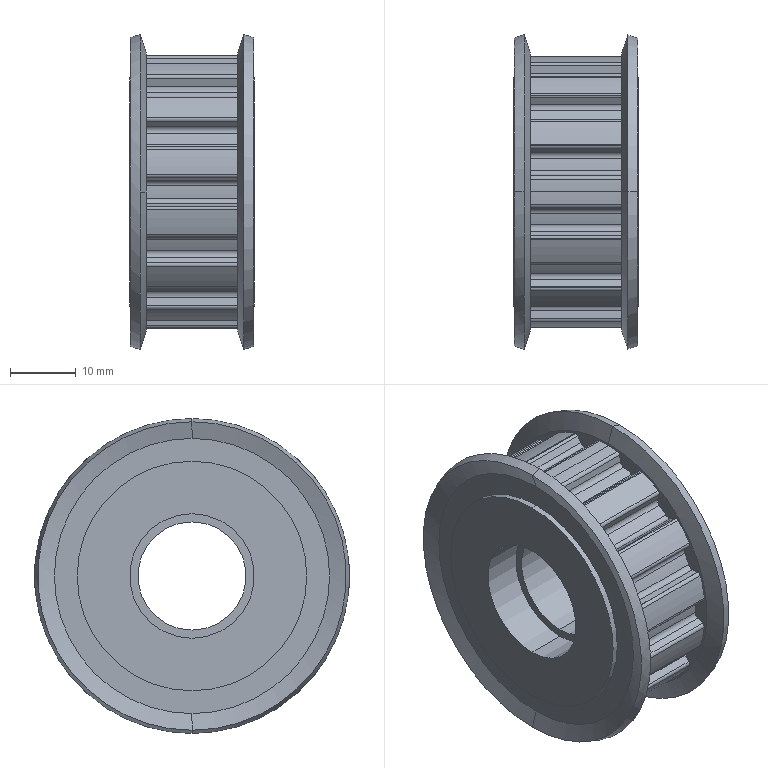Part | NX | features BREP 1 | 1 solid | 155 faces | box 19 x 48 x 48 mm | volume 20074 mm3 | cylinder 107 | plane 36 | cone 12 | commonest cylinder face diameters 1.06 x34 1.72 x34 41.68 x15 37.42 x14 19 x4 35 x4